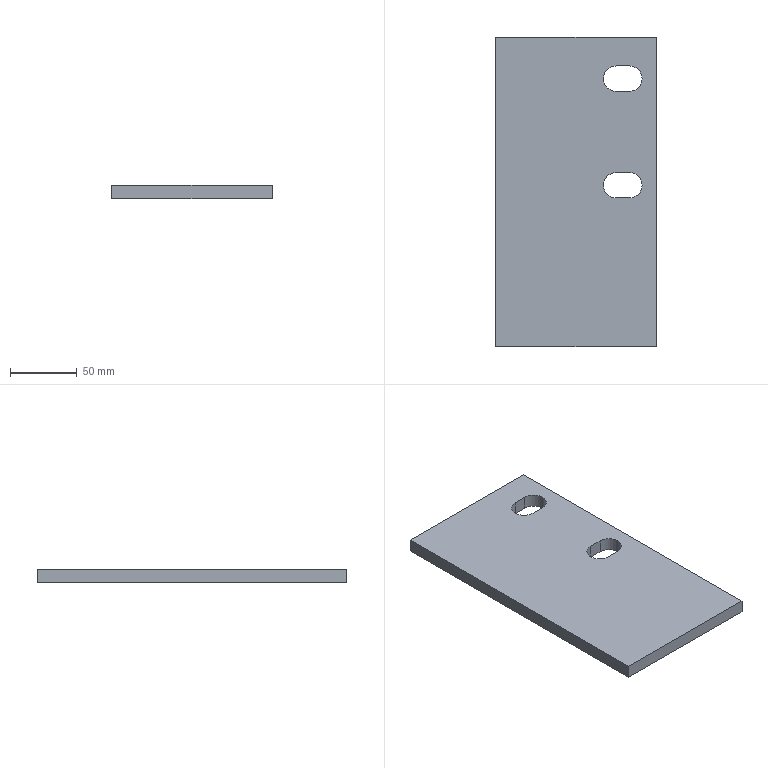Part | STEP file | 粉仓楼梯支撑Plate | 1 solid | 16 faces | box 120 x 232 x 10 mm | volume 268929 mm3 | plane 10 | cylinder 6 | commonest cylinder face diameters 19 x6
STEP:
#1=CARTESIAN_POINT('',(0.,0.,0.));
#2=DIRECTION('',(0.,0.,1.));
#3=DIRECTION('',(1.,0.,0.));
#4=AXIS2_PLACEMENT_3D('',#1,#2,#3);
#5=CARTESIAN_POINT('',(40.,94.5,0.));
#6=VERTEX_POINT('',#5);
#7=CARTESIAN_POINT('',(40.,94.5,10.));
#8=VERTEX_POINT('',#7);
#9=CARTESIAN_POINT('',(40.,94.5,10.));
#10=DIRECTION('',(0.,0.,1.));
#11=VECTOR('',#10,1.);
#12=LINE('',#9,#11);
#13=CARTESIAN_POINT('',(40.,85.,10.));
#14=DIRECTION('',(0.,0.,1.));
#15=DIRECTION('',(1.,0.,0.));
#16=AXIS2_PLACEMENT_3D('',#13,#14,#15);
#17=CYLINDRICAL_SURFACE('',#16,9.5);
#18=CARTESIAN_POINT('',(1.571,0.));
#19=DIRECTION('',(0.,1.));
#20=VECTOR('',#19,1.);
#21=LINE('',#18,#20);
#22=(GEOMETRIC_REPRESENTATION_CONTEXT(2)PARAMETRIC_REPRESENTATION_CONTEXT()REPRESENTATION_CONTEXT('',''));
#23=DEFINITIONAL_REPRESENTATION('',(#21),#22);
#24=PCURVE('',#17,#23);
#25=CARTESIAN_POINT('',(30.,94.5,10.));
#26=DIRECTION('',(0.,1.,0.));
#27=DIRECTION('',(0.,0.,1.));
#28=AXIS2_PLACEMENT_3D('',#25,#26,#27);
#29=PLANE('',#28);
#30=CARTESIAN_POINT('',(0.,10.));
#31=DIRECTION('',(1.,0.));
#32=VECTOR('',#31,1.);
#33=LINE('',#30,#32);
#34=(GEOMETRIC_REPRESENTATION_CONTEXT(2)PARAMETRIC_REPRESENTATION_CONTEXT()REPRESENTATION_CONTEXT('',''));
#35=DEFINITIONAL_REPRESENTATION('',(#33),#34);
#36=PCURVE('',#29,#35);
#37=SURFACE_CURVE('',#12,(#24,#36),.PCURVE_S1.);
#38=EDGE_CURVE('',#6,#8,#37,.T.);
#39=ORIENTED_EDGE('',*,*,#38,.T.);
#40=CARTESIAN_POINT('',(49.5,85.,10.));
#41=VERTEX_POINT('',#40);
#42=CARTESIAN_POINT('',(40.,85.,10.));
#43=DIRECTION('',(0.,0.,1.));
#44=DIRECTION('',(1.,0.,0.));
#45=AXIS2_PLACEMENT_3D('',#42,#43,#44);
#46=CIRCLE('',#45,9.5);
#47=CARTESIAN_POINT('',(0.,0.));
#48=DIRECTION('',(1.,0.));
#49=VECTOR('',#48,1.);
#50=LINE('',#47,#49);
#51=(GEOMETRIC_REPRESENTATION_CONTEXT(2)PARAMETRIC_REPRESENTATION_CONTEXT()REPRESENTATION_CONTEXT('',''));
#52=DEFINITIONAL_REPRESENTATION('',(#50),#51);
#53=PCURVE('',#17,#52);
#54=CARTESIAN_POINT('',(0.,0.,10.));
#55=DIRECTION('',(0.,0.,1.));
#56=DIRECTION('',(1.,0.,0.));
#57=AXIS2_PLACEMENT_3D('',#54,#55,#56);
#58=PLANE('',#57);
#59=CARTESIAN_POINT('',(40.,85.));
#60=DIRECTION('',(1.,0.));
#61=AXIS2_PLACEMENT_2D('',#59,#60);
#62=CIRCLE('',#61,9.5);
#63=(GEOMETRIC_REPRESENTATION_CONTEXT(2)PARAMETRIC_REPRESENTATION_CONTEXT()REPRESENTATION_CONTEXT('',''));
#64=DEFINITIONAL_REPRESENTATION('',(#62),#63);
#65=PCURVE('',#58,#64);
#66=SURFACE_CURVE('',#46,(#53,#65),.PCURVE_S1.);
#67=EDGE_CURVE('',#41,#8,#66,.T.);
#68=ORIENTED_EDGE('',*,*,#67,.F.);
#69=CARTESIAN_POINT('',(49.5,85.,0.));
#70=VERTEX_POINT('',#69);
#71=CARTESIAN_POINT('',(49.5,85.,10.));
#72=DIRECTION('',(0.,0.,1.));
#73=VECTOR('',#72,1.);
#74=LINE('',#71,#73);
#75=CARTESIAN_POINT('',(0.,0.));
#76=DIRECTION('',(0.,1.));
#77=VECTOR('',#76,1.);
#78=LINE('',#75,#77);
#79=(GEOMETRIC_REPRESENTATION_CONTEXT(2)PARAMETRIC_REPRESENTATION_CONTEXT()REPRESENTATION_CONTEXT('',''));
#80=DEFINITIONAL_REPRESENTATION('',(#78),#79);
#81=PCURVE('',#17,#80);
#82=CARTESIAN_POINT('',(40.,85.,10.));
#83=DIRECTION('',(0.,0.,1.));
#84=DIRECTION('',(1.,0.,0.));
#85=AXIS2_PLACEMENT_3D('',#82,#83,#84);
#86=CYLINDRICAL_SURFACE('',#85,9.5);
#87=CARTESIAN_POINT('',(6.283,0.));
#88=DIRECTION('',(0.,1.));
#89=VECTOR('',#88,1.);
#90=LINE('',#87,#89);
#91=(GEOMETRIC_REPRESENTATION_CONTEXT(2)PARAMETRIC_REPRESENTATION_CONTEXT()REPRESENTATION_CONTEXT('',''));
#92=DEFINITIONAL_REPRESENTATION('',(#90),#91);
#93=PCURVE('',#86,#92);
#94=SURFACE_CURVE('',#74,(#81,#93),.PCURVE_S1.);
#95=EDGE_CURVE('',#70,#41,#94,.T.);
#96=ORIENTED_EDGE('',*,*,#95,.F.);
#97=CARTESIAN_POINT('',(40.,85.,0.));
#98=DIRECTION('',(0.,0.,1.));
#99=DIRECTION('',(1.,0.,0.));
#100=AXIS2_PLACEMENT_3D('',#97,#98,#99);
#101=CIRCLE('',#100,9.5);
#102=CARTESIAN_POINT('',(0.,-10.));
#103=DIRECTION('',(1.,0.));
#104=VECTOR('',#103,1.);
#105=LINE('',#102,#104);
#106=(GEOMETRIC_REPRESENTATION_CONTEXT(2)PARAMETRIC_REPRESENTATION_CONTEXT()REPRESENTATION_CONTEXT('',''));
#107=DEFINITIONAL_REPRESENTATION('',(#105),#106);
#108=PCURVE('',#17,#107);
#109=CARTESIAN_POINT('',(0.,0.,0.));
#110=DIRECTION('',(0.,0.,1.));
#111=DIRECTION('',(1.,0.,0.));
#112=AXIS2_PLACEMENT_3D('',#109,#110,#111);
#113=PLANE('',#112);
#114=CARTESIAN_POINT('',(40.,85.));
#115=DIRECTION('',(1.,0.));
#116=AXIS2_PLACEMENT_2D('',#114,#115);
#117=CIRCLE('',#116,9.5);
#118=(GEOMETRIC_REPRESENTATION_CONTEXT(2)PARAMETRIC_REPRESENTATION_CONTEXT()REPRESENTATION_CONTEXT('',''));
#119=DEFINITIONAL_REPRESENTATION('',(#117),#118);
#120=PCURVE('',#113,#119);
#121=SURFACE_CURVE('',#101,(#108,#120),.PCURVE_S1.);
#122=EDGE_CURVE('',#70,#6,#121,.T.);
#123=ORIENTED_EDGE('',*,*,#122,.T.);
#124=EDGE_LOOP('',(#39,#68,#96,#123));
#125=FACE_BOUND('',#124,.F.);
#126=ADVANCED_FACE('',(#125),#17,.F.);
#127=CARTESIAN_POINT('',(40.,14.5,0.));
#128=VERTEX_POINT('',#127);
#129=CARTESIAN_POINT('',(40.,14.5,10.));
#130=VERTEX_POINT('',#129);
#131=CARTESIAN_POINT('',(40.,14.5,10.));
#132=DIRECTION('',(0.,0.,1.));
#133=VECTOR('',#132,1.);
#134=LINE('',#131,#133);
#135=CARTESIAN_POINT('',(40.,5.,10.));
#136=DIRECTION('',(0.,0.,1.));
#137=DIRECTION('',(1.,0.,0.));
#138=AXIS2_PLACEMENT_3D('',#135,#136,#137);
#139=CYLINDRICAL_SURFACE('',#138,9.5);
#140=CARTESIAN_POINT('',(1.571,0.));
#141=DIRECTION('',(0.,1.));
#142=VECTOR('',#141,1.);
#143=LINE('',#140,#142);
#144=(GEOMETRIC_REPRESENTATION_CONTEXT(2)PARAMETRIC_REPRESENTATION_CONTEXT()REPRESENTATION_CONTEXT('',''));
#145=DEFINITIONAL_REPRESENTATION('',(#143),#144);
#146=PCURVE('',#139,#145);
#147=CARTESIAN_POINT('',(30.,14.5,10.));
#148=DIRECTION('',(0.,1.,0.));
#149=DIRECTION('',(0.,0.,1.));
#150=AXIS2_PLACEMENT_3D('',#147,#148,#149);
#151=PLANE('',#150);
#152=CARTESIAN_POINT('',(0.,10.));
#153=DIRECTION('',(1.,0.));
#154=VECTOR('',#153,1.);
#155=LINE('',#152,#154);
#156=(GEOMETRIC_REPRESENTATION_CONTEXT(2)PARAMETRIC_REPRESENTATION_CONTEXT()REPRESENTATION_CONTEXT('',''));
#157=DEFINITIONAL_REPRESENTATION('',(#155),#156);
#158=PCURVE('',#151,#157);
#159=SURFACE_CURVE('',#134,(#146,#158),.PCURVE_S1.);
#160=EDGE_CURVE('',#128,#130,#159,.T.);
#161=ORIENTED_EDGE('',*,*,#160,.T.);
#162=CARTESIAN_POINT('',(49.5,5.,10.));
#163=VERTEX_POINT('',#162);
#164=CARTESIAN_POINT('',(40.,5.,10.));
#165=DIRECTION('',(0.,0.,1.));
#166=DIRECTION('',(1.,0.,0.));
#167=AXIS2_PLACEMENT_3D('',#164,#165,#166);
#168=CIRCLE('',#167,9.5);
#169=CARTESIAN_POINT('',(0.,0.));
#170=DIRECTION('',(1.,0.));
#171=VECTOR('',#170,1.);
#172=LINE('',#169,#171);
#173=(GEOMETRIC_REPRESENTATION_CONTEXT(2)PARAMETRIC_REPRESENTATION_CONTEXT()REPRESENTATION_CONTEXT('',''));
#174=DEFINITIONAL_REPRESENTATION('',(#172),#173);
#175=PCURVE('',#139,#174);
#176=CARTESIAN_POINT('',(40.,5.));
#177=DIRECTION('',(1.,0.));
#178=AXIS2_PLACEMENT_2D('',#176,#177);
#179=CIRCLE('',#178,9.5);
#180=(GEOMETRIC_REPRESENTATION_CONTEXT(2)PARAMETRIC_REPRESENTATION_CONTEXT()REPRESENTATION_CONTEXT('',''));
#181=DEFINITIONAL_REPRESENTATION('',(#179),#180);
#182=PCURVE('',#58,#181);
#183=SURFACE_CURVE('',#168,(#175,#182),.PCURVE_S1.);
#184=EDGE_CURVE('',#163,#130,#183,.T.);
#185=ORIENTED_EDGE('',*,*,#184,.F.);
#186=CARTESIAN_POINT('',(49.5,5.,0.));
#187=VERTEX_POINT('',#186);
#188=CARTESIAN_POINT('',(49.5,5.,10.));
#189=DIRECTION('',(0.,0.,1.));
#190=VECTOR('',#189,1.);
#191=LINE('',#188,#190);
#192=CARTESIAN_POINT('',(0.,0.));
#193=DIRECTION('',(0.,1.));
#194=VECTOR('',#193,1.);
#195=LINE('',#192,#194);
#196=(GEOMETRIC_REPRESENTATION_CONTEXT(2)PARAMETRIC_REPRESENTATION_CONTEXT()REPRESENTATION_CONTEXT('',''));
#197=DEFINITIONAL_REPRESENTATION('',(#195),#196);
#198=PCURVE('',#139,#197);
#199=CARTESIAN_POINT('',(40.,5.,10.));
#200=DIRECTION('',(0.,0.,1.));
#201=DIRECTION('',(1.,0.,0.));
#202=AXIS2_PLACEMENT_3D('',#199,#200,#201);
#203=CYLINDRICAL_SURFACE('',#202,9.5);
#204=CARTESIAN_POINT('',(6.283,0.));
#205=DIRECTION('',(0.,1.));
#206=VECTOR('',#205,1.);
#207=LINE('',#204,#206);
#208=(GEOMETRIC_REPRESENTATION_CONTEXT(2)PARAMETRIC_REPRESENTATION_CONTEXT()REPRESENTATION_CONTEXT('',''));
#209=DEFINITIONAL_REPRESENTATION('',(#207),#208);
#210=PCURVE('',#203,#209);
#211=SURFACE_CURVE('',#191,(#198,#210),.PCURVE_S1.);
#212=EDGE_CURVE('',#187,#163,#211,.T.);
#213=ORIENTED_EDGE('',*,*,#212,.F.);
#214=CARTESIAN_POINT('',(40.,5.,0.));
#215=DIRECTION('',(0.,0.,1.));
#216=DIRECTION('',(1.,0.,0.));
#217=AXIS2_PLACEMENT_3D('',#214,#215,#216);
#218=CIRCLE('',#217,9.5);
#219=CARTESIAN_POINT('',(0.,-10.));
#220=DIRECTION('',(1.,0.));
#221=VECTOR('',#220,1.);
#222=LINE('',#219,#221);
#223=(GEOMETRIC_REPRESENTATION_CONTEXT(2)PARAMETRIC_REPRESENTATION_CONTEXT()REPRESENTATION_CONTEXT('',''));
#224=DEFINITIONAL_REPRESENTATION('',(#222),#223);
#225=PCURVE('',#139,#224);
#226=CARTESIAN_POINT('',(40.,5.));
#227=DIRECTION('',(1.,0.));
#228=AXIS2_PLACEMENT_2D('',#226,#227);
#229=CIRCLE('',#228,9.5);
#230=(GEOMETRIC_REPRESENTATION_CONTEXT(2)PARAMETRIC_REPRESENTATION_CONTEXT()REPRESENTATION_CONTEXT('',''));
#231=DEFINITIONAL_REPRESENTATION('',(#229),#230);
#232=PCURVE('',#113,#231);
#233=SURFACE_CURVE('',#218,(#225,#232),.PCURVE_S1.);
#234=EDGE_CURVE('',#187,#128,#233,.T.);
#235=ORIENTED_EDGE('',*,*,#234,.T.);
#236=EDGE_LOOP('',(#161,#185,#213,#235));
#237=FACE_BOUND('',#236,.F.);
#238=ADVANCED_FACE('',(#237),#139,.F.);
#239=CARTESIAN_POINT('',(60.,-116.,0.));
#240=VERTEX_POINT('',#239);
#241=CARTESIAN_POINT('',(60.,116.,0.));
#242=VERTEX_POINT('',#241);
#243=CARTESIAN_POINT('',(60.,116.,0.));
#244=DIRECTION('',(0.,1.,0.));
#245=VECTOR('',#244,1.);
#246=LINE('',#243,#245);
#247=CARTESIAN_POINT('',(60.,116.,10.));
#248=DIRECTION('',(-1.,0.,0.));
#249=DIRECTION('',(0.,-1.,0.));
#250=AXIS2_PLACEMENT_3D('',#247,#248,#249);
#251=PLANE('',#250);
#252=CARTESIAN_POINT('',(0.,-10.));
#253=DIRECTION('',(-1.,0.));
#254=VECTOR('',#253,1.);
#255=LINE('',#252,#254);
#256=(GEOMETRIC_REPRESENTATION_CONTEXT(2)PARAMETRIC_REPRESENTATION_CONTEXT()REPRESENTATION_CONTEXT('',''));
#257=DEFINITIONAL_REPRESENTATION('',(#255),#256);
#258=PCURVE('',#251,#257);
#259=CARTESIAN_POINT('',(60.,116.));
#260=DIRECTION('',(0.,1.));
#261=VECTOR('',#260,1.);
#262=LINE('',#259,#261);
#263=(GEOMETRIC_REPRESENTATION_CONTEXT(2)PARAMETRIC_REPRESENTATION_CONTEXT()REPRESENTATION_CONTEXT('',''));
#264=DEFINITIONAL_REPRESENTATION('',(#262),#263);
#265=PCURVE('',#113,#264);
#266=SURFACE_CURVE('',#246,(#258,#265),.PCURVE_S1.);
#267=EDGE_CURVE('',#240,#242,#266,.T.);
#268=ORIENTED_EDGE('',*,*,#267,.T.);
#269=CARTESIAN_POINT('',(60.,116.,10.));
#270=VERTEX_POINT('',#269);
#271=CARTESIAN_POINT('',(60.,116.,10.));
#272=DIRECTION('',(0.,0.,-1.));
#273=VECTOR('',#272,1.);
#274=LINE('',#271,#273);
#275=CARTESIAN_POINT('',(0.,0.));
#276=DIRECTION('',(0.,-1.));
#277=VECTOR('',#276,1.);
#278=LINE('',#275,#277);
#279=(GEOMETRIC_REPRESENTATION_CONTEXT(2)PARAMETRIC_REPRESENTATION_CONTEXT()REPRESENTATION_CONTEXT('',''));
#280=DEFINITIONAL_REPRESENTATION('',(#278),#279);
#281=PCURVE('',#251,#280);
#282=CARTESIAN_POINT('',(-60.,116.,10.));
#283=DIRECTION('',(0.,-1.,0.));
#284=DIRECTION('',(1.,0.,0.));
#285=AXIS2_PLACEMENT_3D('',#282,#283,#284);
#286=PLANE('',#285);
#287=CARTESIAN_POINT('',(120.,0.));
#288=DIRECTION('',(0.,-1.));
#289=VECTOR('',#288,1.);
#290=LINE('',#287,#289);
#291=(GEOMETRIC_REPRESENTATION_CONTEXT(2)PARAMETRIC_REPRESENTATION_CONTEXT()REPRESENTATION_CONTEXT('',''));
#292=DEFINITIONAL_REPRESENTATION('',(#290),#291);
#293=PCURVE('',#286,#292);
#294=SURFACE_CURVE('',#274,(#281,#293),.PCURVE_S1.);
#295=EDGE_CURVE('',#270,#242,#294,.T.);
#296=ORIENTED_EDGE('',*,*,#295,.F.);
#297=CARTESIAN_POINT('',(60.,-116.,10.));
#298=VERTEX_POINT('',#297);
#299=CARTESIAN_POINT('',(60.,116.,10.));
#300=DIRECTION('',(0.,1.,0.));
#301=VECTOR('',#300,1.);
#302=LINE('',#299,#301);
#303=CARTESIAN_POINT('',(0.,0.));
#304=DIRECTION('',(-1.,0.));
#305=VECTOR('',#304,1.);
#306=LINE('',#303,#305);
#307=(GEOMETRIC_REPRESENTATION_CONTEXT(2)PARAMETRIC_REPRESENTATION_CONTEXT()REPRESENTATION_CONTEXT('',''));
#308=DEFINITIONAL_REPRESENTATION('',(#306),#307);
#309=PCURVE('',#251,#308);
#310=CARTESIAN_POINT('',(60.,116.));
#311=DIRECTION('',(0.,1.));
#312=VECTOR('',#311,1.);
#313=LINE('',#310,#312);
#314=(GEOMETRIC_REPRESENTATION_CONTEXT(2)PARAMETRIC_REPRESENTATION_CONTEXT()REPRESENTATION_CONTEXT('',''));
#315=DEFINITIONAL_REPRESENTATION('',(#313),#314);
#316=PCURVE('',#58,#315);
#317=SURFACE_CURVE('',#302,(#309,#316),.PCURVE_S1.);
#318=EDGE_CURVE('',#298,#270,#317,.T.);
#319=ORIENTED_EDGE('',*,*,#318,.F.);
#320=CARTESIAN_POINT('',(60.,-116.,10.));
#321=DIRECTION('',(0.,0.,-1.));
#322=VECTOR('',#321,1.);
#323=LINE('',#320,#322);
#324=CARTESIAN_POINT('',(232.,0.));
#325=DIRECTION('',(0.,-1.));
#326=VECTOR('',#325,1.);
#327=LINE('',#324,#326);
#328=(GEOMETRIC_REPRESENTATION_CONTEXT(2)PARAMETRIC_REPRESENTATION_CONTEXT()REPRESENTATION_CONTEXT('',''));
#329=DEFINITIONAL_REPRESENTATION('',(#327),#328);
#330=PCURVE('',#251,#329);
#331=CARTESIAN_POINT('',(-60.,-116.,10.));
#332=DIRECTION('',(0.,1.,0.));
#333=DIRECTION('',(0.,0.,1.));
#334=AXIS2_PLACEMENT_3D('',#331,#332,#333);
#335=PLANE('',#334);
#336=CARTESIAN_POINT('',(0.,120.));
#337=DIRECTION('',(-1.,0.));
#338=VECTOR('',#337,1.);
#339=LINE('',#336,#338);
#340=(GEOMETRIC_REPRESENTATION_CONTEXT(2)PARAMETRIC_REPRESENTATION_CONTEXT()REPRESENTATION_CONTEXT('',''));
#341=DEFINITIONAL_REPRESENTATION('',(#339),#340);
#342=PCURVE('',#335,#341);
#343=SURFACE_CURVE('',#323,(#330,#342),.PCURVE_S1.);
#344=EDGE_CURVE('',#298,#240,#343,.T.);
#345=ORIENTED_EDGE('',*,*,#344,.T.);
#346=EDGE_LOOP('',(#268,#296,#319,#345));
#347=FACE_BOUND('',#346,.T.);
#348=ADVANCED_FACE('',(#347),#251,.F.);
#349=CARTESIAN_POINT('',(-60.,116.,0.));
#350=VERTEX_POINT('',#349);
#351=CARTESIAN_POINT('',(-60.,116.,0.));
#352=DIRECTION('',(-1.,0.,0.));
#353=VECTOR('',#352,1.);
#354=LINE('',#351,#353);
#355=CARTESIAN_POINT('',(0.,-10.));
#356=DIRECTION('',(-1.,0.));
#357=VECTOR('',#356,1.);
#358=LINE('',#355,#357);
#359=(GEOMETRIC_REPRESENTATION_CONTEXT(2)PARAMETRIC_REPRESENTATION_CONTEXT()REPRESENTATION_CONTEXT('',''));
#360=DEFINITIONAL_REPRESENTATION('',(#358),#359);
#361=PCURVE('',#286,#360);
#362=CARTESIAN_POINT('',(-60.,116.));
#363=DIRECTION('',(-1.,0.));
#364=VECTOR('',#363,1.);
#365=LINE('',#362,#364);
#366=(GEOMETRIC_REPRESENTATION_CONTEXT(2)PARAMETRIC_REPRESENTATION_CONTEXT()REPRESENTATION_CONTEXT('',''));
#367=DEFINITIONAL_REPRESENTATION('',(#365),#366);
#368=PCURVE('',#113,#367);
#369=SURFACE_CURVE('',#354,(#361,#368),.PCURVE_S1.);
#370=EDGE_CURVE('',#242,#350,#369,.T.);
#371=ORIENTED_EDGE('',*,*,#370,.T.);
#372=CARTESIAN_POINT('',(-60.,116.,10.));
#373=VERTEX_POINT('',#372);
#374=CARTESIAN_POINT('',(-60.,116.,10.));
#375=DIRECTION('',(0.,0.,-1.));
#376=VECTOR('',#375,1.);
#377=LINE('',#374,#376);
#378=CARTESIAN_POINT('',(0.,0.));
#379=DIRECTION('',(0.,-1.));
#380=VECTOR('',#379,1.);
#381=LINE('',#378,#380);
#382=(GEOMETRIC_REPRESENTATION_CONTEXT(2)PARAMETRIC_REPRESENTATION_CONTEXT()REPRESENTATION_CONTEXT('',''));
#383=DEFINITIONAL_REPRESENTATION('',(#381),#382);
#384=PCURVE('',#286,#383);
#385=CARTESIAN_POINT('',(-60.,116.,10.));
#386=DIRECTION('',(1.,0.,0.));
#387=DIRECTION('',(0.,1.,0.));
#388=AXIS2_PLACEMENT_3D('',#385,#386,#387);
#389=PLANE('',#388);
#390=CARTESIAN_POINT('',(0.,0.));
#391=DIRECTION('',(0.,-1.));
#392=VECTOR('',#391,1.);
#393=LINE('',#390,#392);
#394=(GEOMETRIC_REPRESENTATION_CONTEXT(2)PARAMETRIC_REPRESENTATION_CONTEXT()REPRESENTATION_CONTEXT('',''));
#395=DEFINITIONAL_REPRESENTATION('',(#393),#394);
#396=PCURVE('',#389,#395);
#397=SURFACE_CURVE('',#377,(#384,#396),.PCURVE_S1.);
#398=EDGE_CURVE('',#373,#350,#397,.T.);
#399=ORIENTED_EDGE('',*,*,#398,.F.);
#400=CARTESIAN_POINT('',(-60.,116.,10.));
#401=DIRECTION('',(-1.,0.,0.));
#402=VECTOR('',#401,1.);
#403=LINE('',#400,#402);
#404=CARTESIAN_POINT('',(0.,0.));
#405=DIRECTION('',(-1.,0.));
#406=VECTOR('',#405,1.);
#407=LINE('',#404,#406);
#408=(GEOMETRIC_REPRESENTATION_CONTEXT(2)PARAMETRIC_REPRESENTATION_CONTEXT()REPRESENTATION_CONTEXT('',''));
#409=DEFINITIONAL_REPRESENTATION('',(#407),#408);
#410=PCURVE('',#286,#409);
#411=CARTESIAN_POINT('',(-60.,116.));
#412=DIRECTION('',(-1.,0.));
#413=VECTOR('',#412,1.);
#414=LINE('',#411,#413);
#415=(GEOMETRIC_REPRESENTATION_CONTEXT(2)PARAMETRIC_REPRESENTATION_CONTEXT()REPRESENTATION_CONTEXT('',''));
#416=DEFINITIONAL_REPRESENTATION('',(#414),#415);
#417=PCURVE('',#58,#416);
#418=SURFACE_CURVE('',#403,(#410,#417),.PCURVE_S1.);
#419=EDGE_CURVE('',#270,#373,#418,.T.);
#420=ORIENTED_EDGE('',*,*,#419,.F.);
#421=ORIENTED_EDGE('',*,*,#295,.T.);
#422=EDGE_LOOP('',(#371,#399,#420,#421));
#423=FACE_BOUND('',#422,.T.);
#424=ADVANCED_FACE('',(#423),#286,.F.);
#425=CARTESIAN_POINT('',(-60.,-116.,0.));
#426=VERTEX_POINT('',#425);
#427=CARTESIAN_POINT('',(-60.,116.,0.));
#428=DIRECTION('',(0.,-1.,0.));
#429=VECTOR('',#428,1.);
#430=LINE('',#427,#429);
#431=CARTESIAN_POINT('',(0.,-10.));
#432=DIRECTION('',(-1.,0.));
#433=VECTOR('',#432,1.);
#434=LINE('',#431,#433);
#435=(GEOMETRIC_REPRESENTATION_CONTEXT(2)PARAMETRIC_REPRESENTATION_CONTEXT()REPRESENTATION_CONTEXT('',''));
#436=DEFINITIONAL_REPRESENTATION('',(#434),#435);
#437=PCURVE('',#389,#436);
#438=CARTESIAN_POINT('',(-60.,116.));
#439=DIRECTION('',(0.,-1.));
#440=VECTOR('',#439,1.);
#441=LINE('',#438,#440);
#442=(GEOMETRIC_REPRESENTATION_CONTEXT(2)PARAMETRIC_REPRESENTATION_CONTEXT()REPRESENTATION_CONTEXT('',''));
#443=DEFINITIONAL_REPRESENTATION('',(#441),#442);
#444=PCURVE('',#113,#443);
#445=SURFACE_CURVE('',#430,(#437,#444),.PCURVE_S1.);
#446=EDGE_CURVE('',#350,#426,#445,.T.);
#447=ORIENTED_EDGE('',*,*,#446,.T.);
#448=CARTESIAN_POINT('',(-60.,-116.,10.));
#449=VERTEX_POINT('',#448);
#450=CARTESIAN_POINT('',(-60.,-116.,10.));
#451=DIRECTION('',(0.,0.,-1.));
#452=VECTOR('',#451,1.);
#453=LINE('',#450,#452);
#454=CARTESIAN_POINT('',(-232.,0.));
#455=DIRECTION('',(0.,-1.));
#456=VECTOR('',#455,1.);
#457=LINE('',#454,#456);
#458=(GEOMETRIC_REPRESENTATION_CONTEXT(2)PARAMETRIC_REPRESENTATION_CONTEXT()REPRESENTATION_CONTEXT('',''));
#459=DEFINITIONAL_REPRESENTATION('',(#457),#458);
#460=PCURVE('',#389,#459);
#461=CARTESIAN_POINT('',(0.,0.));
#462=DIRECTION('',(-1.,0.));
#463=VECTOR('',#462,1.);
#464=LINE('',#461,#463);
#465=(GEOMETRIC_REPRESENTATION_CONTEXT(2)PARAMETRIC_REPRESENTATION_CONTEXT()REPRESENTATION_CONTEXT('',''));
#466=DEFINITIONAL_REPRESENTATION('',(#464),#465);
#467=PCURVE('',#335,#466);
#468=SURFACE_CURVE('',#453,(#460,#467),.PCURVE_S1.);
#469=EDGE_CURVE('',#449,#426,#468,.T.);
#470=ORIENTED_EDGE('',*,*,#469,.F.);
#471=CARTESIAN_POINT('',(-60.,116.,10.));
#472=DIRECTION('',(0.,-1.,0.));
#473=VECTOR('',#472,1.);
#474=LINE('',#471,#473);
#475=CARTESIAN_POINT('',(0.,0.));
#476=DIRECTION('',(-1.,0.));
#477=VECTOR('',#476,1.);
#478=LINE('',#475,#477);
#479=(GEOMETRIC_REPRESENTATION_CONTEXT(2)PARAMETRIC_REPRESENTATION_CONTEXT()REPRESENTATION_CONTEXT('',''));
#480=DEFINITIONAL_REPRESENTATION('',(#478),#479);
#481=PCURVE('',#389,#480);
#482=CARTESIAN_POINT('',(-60.,116.));
#483=DIRECTION('',(0.,-1.));
#484=VECTOR('',#483,1.);
#485=LINE('',#482,#484);
#486=(GEOMETRIC_REPRESENTATION_CONTEXT(2)PARAMETRIC_REPRESENTATION_CONTEXT()REPRESENTATION_CONTEXT('',''));
#487=DEFINITIONAL_REPRESENTATION('',(#485),#486);
#488=PCURVE('',#58,#487);
#489=SURFACE_CURVE('',#474,(#481,#488),.PCURVE_S1.);
#490=EDGE_CURVE('',#373,#449,#489,.T.);
#491=ORIENTED_EDGE('',*,*,#490,.F.);
#492=ORIENTED_EDGE('',*,*,#398,.T.);
#493=EDGE_LOOP('',(#447,#470,#491,#492));
#494=FACE_BOUND('',#493,.T.);
#495=ADVANCED_FACE('',(#494),#389,.F.);
#496=CARTESIAN_POINT('',(-60.,-116.,0.));
#497=DIRECTION('',(1.,0.,0.));
#498=VECTOR('',#497,1.);
#499=LINE('',#496,#498);
#500=CARTESIAN_POINT('',(-10.,0.));
#501=DIRECTION('',(0.,1.));
#502=VECTOR('',#501,1.);
#503=LINE('',#500,#502);
#504=(GEOMETRIC_REPRESENTATION_CONTEXT(2)PARAMETRIC_REPRESENTATION_CONTEXT()REPRESENTATION_CONTEXT('',''));
#505=DEFINITIONAL_REPRESENTATION('',(#503),#504);
#506=PCURVE('',#335,#505);
#507=CARTESIAN_POINT('',(-60.,-116.));
#508=DIRECTION('',(1.,0.));
#509=VECTOR('',#508,1.);
#510=LINE('',#507,#509);
#511=(GEOMETRIC_REPRESENTATION_CONTEXT(2)PARAMETRIC_REPRESENTATION_CONTEXT()REPRESENTATION_CONTEXT('',''));
#512=DEFINITIONAL_REPRESENTATION('',(#510),#511);
#513=PCURVE('',#113,#512);
#514=SURFACE_CURVE('',#499,(#506,#513),.PCURVE_S1.);
#515=EDGE_CURVE('',#426,#240,#514,.T.);
#516=ORIENTED_EDGE('',*,*,#515,.T.);
#517=ORIENTED_EDGE('',*,*,#344,.F.);
#518=CARTESIAN_POINT('',(-60.,-116.,10.));
#519=DIRECTION('',(1.,0.,0.));
#520=VECTOR('',#519,1.);
#521=LINE('',#518,#520);
#522=CARTESIAN_POINT('',(0.,0.));
#523=DIRECTION('',(0.,1.));
#524=VECTOR('',#523,1.);
#525=LINE('',#522,#524);
#526=(GEOMETRIC_REPRESENTATION_CONTEXT(2)PARAMETRIC_REPRESENTATION_CONTEXT()REPRESENTATION_CONTEXT('',''));
#527=DEFINITIONAL_REPRESENTATION('',(#525),#526);
#528=PCURVE('',#335,#527);
#529=CARTESIAN_POINT('',(-60.,-116.));
#530=DIRECTION('',(1.,0.));
#531=VECTOR('',#530,1.);
#532=LINE('',#529,#531);
#533=(GEOMETRIC_REPRESENTATION_CONTEXT(2)PARAMETRIC_REPRESENTATION_CONTEXT()REPRESENTATION_CONTEXT('',''));
#534=DEFINITIONAL_REPRESENTATION('',(#532),#533);
#535=PCURVE('',#58,#534);
#536=SURFACE_CURVE('',#521,(#528,#535),.PCURVE_S1.);
#537=EDGE_CURVE('',#449,#298,#536,.T.);
#538=ORIENTED_EDGE('',*,*,#537,.F.);
#539=ORIENTED_EDGE('',*,*,#469,.T.);
#540=EDGE_LOOP('',(#516,#517,#538,#539));
#541=FACE_BOUND('',#540,.T.);
#542=ADVANCED_FACE('',(#541),#335,.F.);
#543=CARTESIAN_POINT('',(30.,94.5,10.));
#544=VERTEX_POINT('',#543);
#545=CARTESIAN_POINT('',(30.,75.5,10.));
#546=VERTEX_POINT('',#545);
#547=CARTESIAN_POINT('',(30.,85.,10.));
#548=DIRECTION('',(0.,0.,1.));
#549=DIRECTION('',(1.,0.,0.));
#550=AXIS2_PLACEMENT_3D('',#547,#548,#549);
#551=CIRCLE('',#550,9.5);
#552=CARTESIAN_POINT('',(30.,85.));
#553=DIRECTION('',(1.,0.));
#554=AXIS2_PLACEMENT_2D('',#552,#553);
#555=CIRCLE('',#554,9.5);
#556=(GEOMETRIC_REPRESENTATION_CONTEXT(2)PARAMETRIC_REPRESENTATION_CONTEXT()REPRESENTATION_CONTEXT('',''));
#557=DEFINITIONAL_REPRESENTATION('',(#555),#556);
#558=PCURVE('',#58,#557);
#559=CARTESIAN_POINT('',(30.,85.,10.));
#560=DIRECTION('',(0.,0.,1.));
#561=DIRECTION('',(1.,0.,0.));
#562=AXIS2_PLACEMENT_3D('',#559,#560,#561);
#563=CYLINDRICAL_SURFACE('',#562,9.5);
#564=CARTESIAN_POINT('',(0.,0.));
#565=DIRECTION('',(1.,0.));
#566=VECTOR('',#565,1.);
#567=LINE('',#564,#566);
#568=(GEOMETRIC_REPRESENTATION_CONTEXT(2)PARAMETRIC_REPRESENTATION_CONTEXT()REPRESENTATION_CONTEXT('',''));
#569=DEFINITIONAL_REPRESENTATION('',(#567),#568);
#570=PCURVE('',#563,#569);
#571=SURFACE_CURVE('',#551,(#558,#570),.PCURVE_S1.);
#572=EDGE_CURVE('',#544,#546,#571,.T.);
#573=ORIENTED_EDGE('',*,*,#572,.F.);
#574=CARTESIAN_POINT('',(30.,94.5,10.));
#575=DIRECTION('',(1.,0.,0.));
#576=VECTOR('',#575,1.);
#577=LINE('',#574,#576);
#578=CARTESIAN_POINT('',(30.,94.5));
#579=DIRECTION('',(1.,0.));
#580=VECTOR('',#579,1.);
#581=LINE('',#578,#580);
#582=(GEOMETRIC_REPRESENTATION_CONTEXT(2)PARAMETRIC_REPRESENTATION_CONTEXT()REPRESENTATION_CONTEXT('',''));
#583=DEFINITIONAL_REPRESENTATION('',(#581),#582);
#584=PCURVE('',#58,#583);
#585=CARTESIAN_POINT('',(0.,0.));
#586=DIRECTION('',(0.,1.));
#587=VECTOR('',#586,1.);
#588=LINE('',#585,#587);
#589=(GEOMETRIC_REPRESENTATION_CONTEXT(2)PARAMETRIC_REPRESENTATION_CONTEXT()REPRESENTATION_CONTEXT('',''));
#590=DEFINITIONAL_REPRESENTATION('',(#588),#589);
#591=PCURVE('',#29,#590);
#592=SURFACE_CURVE('',#577,(#584,#591),.PCURVE_S1.);
#593=EDGE_CURVE('',#544,#8,#592,.T.);
#594=ORIENTED_EDGE('',*,*,#593,.T.);
#595=ORIENTED_EDGE('',*,*,#67,.F.);
#596=CARTESIAN_POINT('',(40.,75.5,10.));
#597=VERTEX_POINT('',#596);
#598=CARTESIAN_POINT('',(40.,85.,10.));
#599=DIRECTION('',(0.,0.,1.));
#600=DIRECTION('',(1.,0.,0.));
#601=AXIS2_PLACEMENT_3D('',#598,#599,#600);
#602=CIRCLE('',#601,9.5);
#603=CARTESIAN_POINT('',(40.,85.));
#604=DIRECTION('',(1.,0.));
#605=AXIS2_PLACEMENT_2D('',#603,#604);
#606=CIRCLE('',#605,9.5);
#607=(GEOMETRIC_REPRESENTATION_CONTEXT(2)PARAMETRIC_REPRESENTATION_CONTEXT()REPRESENTATION_CONTEXT('',''));
#608=DEFINITIONAL_REPRESENTATION('',(#606),#607);
#609=PCURVE('',#58,#608);
#610=CARTESIAN_POINT('',(0.,0.));
#611=DIRECTION('',(1.,0.));
#612=VECTOR('',#611,1.);
#613=LINE('',#610,#612);
#614=(GEOMETRIC_REPRESENTATION_CONTEXT(2)PARAMETRIC_REPRESENTATION_CONTEXT()REPRESENTATION_CONTEXT('',''));
#615=DEFINITIONAL_REPRESENTATION('',(#613),#614);
#616=PCURVE('',#86,#615);
#617=SURFACE_CURVE('',#602,(#609,#616),.PCURVE_S1.);
#618=EDGE_CURVE('',#597,#41,#617,.T.);
#619=ORIENTED_EDGE('',*,*,#618,.F.);
#620=CARTESIAN_POINT('',(30.,75.5,10.));
#621=DIRECTION('',(1.,0.,0.));
#622=VECTOR('',#621,1.);
#623=LINE('',#620,#622);
#624=CARTESIAN_POINT('',(30.,75.5));
#625=DIRECTION('',(1.,0.));
#626=VECTOR('',#625,1.);
#627=LINE('',#624,#626);
#628=(GEOMETRIC_REPRESENTATION_CONTEXT(2)PARAMETRIC_REPRESENTATION_CONTEXT()REPRESENTATION_CONTEXT('',''));
#629=DEFINITIONAL_REPRESENTATION('',(#627),#628);
#630=PCURVE('',#58,#629);
#631=CARTESIAN_POINT('',(30.,75.5,10.));
#632=DIRECTION('',(0.,-1.,0.));
#633=DIRECTION('',(0.,0.,-1.));
#634=AXIS2_PLACEMENT_3D('',#631,#632,#633);
#635=PLANE('',#634);
#636=CARTESIAN_POINT('',(0.,0.));
#637=DIRECTION('',(0.,1.));
#638=VECTOR('',#637,1.);
#639=LINE('',#636,#638);
#640=(GEOMETRIC_REPRESENTATION_CONTEXT(2)PARAMETRIC_REPRESENTATION_CONTEXT()REPRESENTATION_CONTEXT('',''));
#641=DEFINITIONAL_REPRESENTATION('',(#639),#640);
#642=PCURVE('',#635,#641);
#643=SURFACE_CURVE('',#623,(#630,#642),.PCURVE_S1.);
#644=EDGE_CURVE('',#546,#597,#643,.T.);
#645=ORIENTED_EDGE('',*,*,#644,.F.);
#646=EDGE_LOOP('',(#573,#594,#595,#619,#645));
#647=FACE_BOUND('',#646,.T.);
#648=CARTESIAN_POINT('',(30.,-4.5,10.));
#649=VERTEX_POINT('',#648);
#650=CARTESIAN_POINT('',(40.,-4.5,10.));
#651=VERTEX_POINT('',#650);
#652=CARTESIAN_POINT('',(30.,-4.5,10.));
#653=DIRECTION('',(1.,0.,0.));
#654=VECTOR('',#653,1.);
#655=LINE('',#652,#654);
#656=CARTESIAN_POINT('',(30.,-4.5));
#657=DIRECTION('',(1.,0.));
#658=VECTOR('',#657,1.);
#659=LINE('',#656,#658);
#660=(GEOMETRIC_REPRESENTATION_CONTEXT(2)PARAMETRIC_REPRESENTATION_CONTEXT()REPRESENTATION_CONTEXT('',''));
#661=DEFINITIONAL_REPRESENTATION('',(#659),#660);
#662=PCURVE('',#58,#661);
#663=CARTESIAN_POINT('',(30.,-4.5,10.));
#664=DIRECTION('',(0.,-1.,0.));
#665=DIRECTION('',(0.,0.,-1.));
#666=AXIS2_PLACEMENT_3D('',#663,#664,#665);
#667=PLANE('',#666);
#668=CARTESIAN_POINT('',(0.,0.));
#669=DIRECTION('',(0.,1.));
#670=VECTOR('',#669,1.);
#671=LINE('',#668,#670);
#672=(GEOMETRIC_REPRESENTATION_CONTEXT(2)PARAMETRIC_REPRESENTATION_CONTEXT()REPRESENTATION_CONTEXT('',''));
#673=DEFINITIONAL_REPRESENTATION('',(#671),#672);
#674=PCURVE('',#667,#673);
#675=SURFACE_CURVE('',#655,(#662,#674),.PCURVE_S1.);
#676=EDGE_CURVE('',#649,#651,#675,.T.);
#677=ORIENTED_EDGE('',*,*,#676,.F.);
#678=CARTESIAN_POINT('',(30.,14.5,10.));
#679=VERTEX_POINT('',#678);
#680=CARTESIAN_POINT('',(30.,5.,10.));
#681=DIRECTION('',(0.,0.,1.));
#682=DIRECTION('',(1.,0.,0.));
#683=AXIS2_PLACEMENT_3D('',#680,#681,#682);
#684=CIRCLE('',#683,9.5);
#685=CARTESIAN_POINT('',(30.,5.));
#686=DIRECTION('',(1.,0.));
#687=AXIS2_PLACEMENT_2D('',#685,#686);
#688=CIRCLE('',#687,9.5);
#689=(GEOMETRIC_REPRESENTATION_CONTEXT(2)PARAMETRIC_REPRESENTATION_CONTEXT()REPRESENTATION_CONTEXT('',''));
#690=DEFINITIONAL_REPRESENTATION('',(#688),#689);
#691=PCURVE('',#58,#690);
#692=CARTESIAN_POINT('',(30.,5.,10.));
#693=DIRECTION('',(0.,0.,1.));
#694=DIRECTION('',(1.,0.,0.));
#695=AXIS2_PLACEMENT_3D('',#692,#693,#694);
#696=CYLINDRICAL_SURFACE('',#695,9.5);
#697=CARTESIAN_POINT('',(0.,0.));
#698=DIRECTION('',(1.,0.));
#699=VECTOR('',#698,1.);
#700=LINE('',#697,#699);
#701=(GEOMETRIC_REPRESENTATION_CONTEXT(2)PARAMETRIC_REPRESENTATION_CONTEXT()REPRESENTATION_CONTEXT('',''));
#702=DEFINITIONAL_REPRESENTATION('',(#700),#701);
#703=PCURVE('',#696,#702);
#704=SURFACE_CURVE('',#684,(#691,#703),.PCURVE_S1.);
#705=EDGE_CURVE('',#679,#649,#704,.T.);
#706=ORIENTED_EDGE('',*,*,#705,.F.);
#707=CARTESIAN_POINT('',(30.,14.5,10.));
#708=DIRECTION('',(1.,0.,0.));
#709=VECTOR('',#708,1.);
#710=LINE('',#707,#709);
#711=CARTESIAN_POINT('',(30.,14.5));
#712=DIRECTION('',(1.,0.));
#713=VECTOR('',#712,1.);
#714=LINE('',#711,#713);
#715=(GEOMETRIC_REPRESENTATION_CONTEXT(2)PARAMETRIC_REPRESENTATION_CONTEXT()REPRESENTATION_CONTEXT('',''));
#716=DEFINITIONAL_REPRESENTATION('',(#714),#715);
#717=PCURVE('',#58,#716);
#718=CARTESIAN_POINT('',(0.,0.));
#719=DIRECTION('',(0.,1.));
#720=VECTOR('',#719,1.);
#721=LINE('',#718,#720);
#722=(GEOMETRIC_REPRESENTATION_CONTEXT(2)PARAMETRIC_REPRESENTATION_CONTEXT()REPRESENTATION_CONTEXT('',''));
#723=DEFINITIONAL_REPRESENTATION('',(#721),#722);
#724=PCURVE('',#151,#723);
#725=SURFACE_CURVE('',#710,(#717,#724),.PCURVE_S1.);
#726=EDGE_CURVE('',#679,#130,#725,.T.);
#727=ORIENTED_EDGE('',*,*,#726,.T.);
#728=ORIENTED_EDGE('',*,*,#184,.F.);
#729=CARTESIAN_POINT('',(40.,5.,10.));
#730=DIRECTION('',(0.,0.,1.));
#731=DIRECTION('',(1.,0.,0.));
#732=AXIS2_PLACEMENT_3D('',#729,#730,#731);
#733=CIRCLE('',#732,9.5);
#734=CARTESIAN_POINT('',(40.,5.));
#735=DIRECTION('',(1.,0.));
#736=AXIS2_PLACEMENT_2D('',#734,#735);
#737=CIRCLE('',#736,9.5);
#738=(GEOMETRIC_REPRESENTATION_CONTEXT(2)PARAMETRIC_REPRESENTATION_CONTEXT()REPRESENTATION_CONTEXT('',''));
#739=DEFINITIONAL_REPRESENTATION('',(#737),#738);
#740=PCURVE('',#58,#739);
#741=CARTESIAN_POINT('',(0.,0.));
#742=DIRECTION('',(1.,0.));
#743=VECTOR('',#742,1.);
#744=LINE('',#741,#743);
#745=(GEOMETRIC_REPRESENTATION_CONTEXT(2)PARAMETRIC_REPRESENTATION_CONTEXT()REPRESENTATION_CONTEXT('',''));
#746=DEFINITIONAL_REPRESENTATION('',(#744),#745);
#747=PCURVE('',#203,#746);
#748=SURFACE_CURVE('',#733,(#740,#747),.PCURVE_S1.);
#749=EDGE_CURVE('',#651,#163,#748,.T.);
#750=ORIENTED_EDGE('',*,*,#749,.F.);
#751=EDGE_LOOP('',(#677,#706,#727,#728,#750));
#752=FACE_BOUND('',#751,.T.);
#753=ORIENTED_EDGE('',*,*,#318,.T.);
#754=ORIENTED_EDGE('',*,*,#419,.T.);
#755=ORIENTED_EDGE('',*,*,#490,.T.);
#756=ORIENTED_EDGE('',*,*,#537,.T.);
#757=EDGE_LOOP('',(#753,#754,#755,#756));
#758=FACE_BOUND('',#757,.T.);
#759=ADVANCED_FACE('',(#647,#752,#758),#58,.T.);
#760=CARTESIAN_POINT('',(30.,94.5,0.));
#761=VERTEX_POINT('',#760);
#762=CARTESIAN_POINT('',(0.,94.5,0.));
#763=DIRECTION('',(-1.,0.,0.));
#764=VECTOR('',#763,1.);
#765=LINE('',#762,#764);
#766=CARTESIAN_POINT('',(0.,94.5));
#767=DIRECTION('',(-1.,0.));
#768=VECTOR('',#767,1.);
#769=LINE('',#766,#768);
#770=(GEOMETRIC_REPRESENTATION_CONTEXT(2)PARAMETRIC_REPRESENTATION_CONTEXT()REPRESENTATION_CONTEXT('',''));
#771=DEFINITIONAL_REPRESENTATION('',(#769),#770);
#772=PCURVE('',#113,#771);
#773=CARTESIAN_POINT('',(-10.,-30.));
#774=DIRECTION('',(0.,-1.));
#775=VECTOR('',#774,1.);
#776=LINE('',#773,#775);
#777=(GEOMETRIC_REPRESENTATION_CONTEXT(2)PARAMETRIC_REPRESENTATION_CONTEXT()REPRESENTATION_CONTEXT('',''));
#778=DEFINITIONAL_REPRESENTATION('',(#776),#777);
#779=PCURVE('',#29,#778);
#780=SURFACE_CURVE('',#765,(#772,#779),.PCURVE_S1.);
#781=EDGE_CURVE('',#6,#761,#780,.T.);
#782=ORIENTED_EDGE('',*,*,#781,.T.);
#783=CARTESIAN_POINT('',(30.,75.5,0.));
#784=VERTEX_POINT('',#783);
#785=CARTESIAN_POINT('',(30.,85.,0.));
#786=DIRECTION('',(0.,0.,1.));
#787=DIRECTION('',(1.,0.,0.));
#788=AXIS2_PLACEMENT_3D('',#785,#786,#787);
#789=CIRCLE('',#788,9.5);
#790=CARTESIAN_POINT('',(30.,85.));
#791=DIRECTION('',(1.,0.));
#792=AXIS2_PLACEMENT_2D('',#790,#791);
#793=CIRCLE('',#792,9.5);
#794=(GEOMETRIC_REPRESENTATION_CONTEXT(2)PARAMETRIC_REPRESENTATION_CONTEXT()REPRESENTATION_CONTEXT('',''));
#795=DEFINITIONAL_REPRESENTATION('',(#793),#794);
#796=PCURVE('',#113,#795);
#797=CARTESIAN_POINT('',(0.,-10.));
#798=DIRECTION('',(1.,0.));
#799=VECTOR('',#798,1.);
#800=LINE('',#797,#799);
#801=(GEOMETRIC_REPRESENTATION_CONTEXT(2)PARAMETRIC_REPRESENTATION_CONTEXT()REPRESENTATION_CONTEXT('',''));
#802=DEFINITIONAL_REPRESENTATION('',(#800),#801);
#803=PCURVE('',#563,#802);
#804=SURFACE_CURVE('',#789,(#796,#803),.PCURVE_S1.);
#805=EDGE_CURVE('',#761,#784,#804,.T.);
#806=ORIENTED_EDGE('',*,*,#805,.T.);
#807=CARTESIAN_POINT('',(40.,75.5,0.));
#808=VERTEX_POINT('',#807);
#809=CARTESIAN_POINT('',(0.,75.5,0.));
#810=DIRECTION('',(1.,0.,0.));
#811=VECTOR('',#810,1.);
#812=LINE('',#809,#811);
#813=CARTESIAN_POINT('',(0.,75.5));
#814=DIRECTION('',(1.,0.));
#815=VECTOR('',#814,1.);
#816=LINE('',#813,#815);
#817=(GEOMETRIC_REPRESENTATION_CONTEXT(2)PARAMETRIC_REPRESENTATION_CONTEXT()REPRESENTATION_CONTEXT('',''));
#818=DEFINITIONAL_REPRESENTATION('',(#816),#817);
#819=PCURVE('',#113,#818);
#820=CARTESIAN_POINT('',(10.,-30.));
#821=DIRECTION('',(0.,1.));
#822=VECTOR('',#821,1.);
#823=LINE('',#820,#822);
#824=(GEOMETRIC_REPRESENTATION_CONTEXT(2)PARAMETRIC_REPRESENTATION_CONTEXT()REPRESENTATION_CONTEXT('',''));
#825=DEFINITIONAL_REPRESENTATION('',(#823),#824);
#826=PCURVE('',#635,#825);
#827=SURFACE_CURVE('',#812,(#819,#826),.PCURVE_S1.);
#828=EDGE_CURVE('',#784,#808,#827,.T.);
#829=ORIENTED_EDGE('',*,*,#828,.T.);
#830=CARTESIAN_POINT('',(40.,85.,0.));
#831=DIRECTION('',(0.,0.,1.));
#832=DIRECTION('',(1.,0.,0.));
#833=AXIS2_PLACEMENT_3D('',#830,#831,#832);
#834=CIRCLE('',#833,9.5);
#835=CARTESIAN_POINT('',(40.,85.));
#836=DIRECTION('',(1.,0.));
#837=AXIS2_PLACEMENT_2D('',#835,#836);
#838=CIRCLE('',#837,9.5);
#839=(GEOMETRIC_REPRESENTATION_CONTEXT(2)PARAMETRIC_REPRESENTATION_CONTEXT()REPRESENTATION_CONTEXT('',''));
#840=DEFINITIONAL_REPRESENTATION('',(#838),#839);
#841=PCURVE('',#113,#840);
#842=CARTESIAN_POINT('',(0.,-10.));
#843=DIRECTION('',(1.,0.));
#844=VECTOR('',#843,1.);
#845=LINE('',#842,#844);
#846=(GEOMETRIC_REPRESENTATION_CONTEXT(2)PARAMETRIC_REPRESENTATION_CONTEXT()REPRESENTATION_CONTEXT('',''));
#847=DEFINITIONAL_REPRESENTATION('',(#845),#846);
#848=PCURVE('',#86,#847);
#849=SURFACE_CURVE('',#834,(#841,#848),.PCURVE_S1.);
#850=EDGE_CURVE('',#808,#70,#849,.T.);
#851=ORIENTED_EDGE('',*,*,#850,.T.);
#852=ORIENTED_EDGE('',*,*,#122,.T.);
#853=EDGE_LOOP('',(#782,#806,#829,#851,#852));
#854=FACE_BOUND('',#853,.T.);
#855=CARTESIAN_POINT('',(40.,-4.5,0.));
#856=VERTEX_POINT('',#855);
#857=CARTESIAN_POINT('',(40.,5.,0.));
#858=DIRECTION('',(0.,0.,1.));
#859=DIRECTION('',(1.,0.,0.));
#860=AXIS2_PLACEMENT_3D('',#857,#858,#859);
#861=CIRCLE('',#860,9.5);
#862=CARTESIAN_POINT('',(40.,5.));
#863=DIRECTION('',(1.,0.));
#864=AXIS2_PLACEMENT_2D('',#862,#863);
#865=CIRCLE('',#864,9.5);
#866=(GEOMETRIC_REPRESENTATION_CONTEXT(2)PARAMETRIC_REPRESENTATION_CONTEXT()REPRESENTATION_CONTEXT('',''));
#867=DEFINITIONAL_REPRESENTATION('',(#865),#866);
#868=PCURVE('',#113,#867);
#869=CARTESIAN_POINT('',(0.,-10.));
#870=DIRECTION('',(1.,0.));
#871=VECTOR('',#870,1.);
#872=LINE('',#869,#871);
#873=(GEOMETRIC_REPRESENTATION_CONTEXT(2)PARAMETRIC_REPRESENTATION_CONTEXT()REPRESENTATION_CONTEXT('',''));
#874=DEFINITIONAL_REPRESENTATION('',(#872),#873);
#875=PCURVE('',#203,#874);
#876=SURFACE_CURVE('',#861,(#868,#875),.PCURVE_S1.);
#877=EDGE_CURVE('',#856,#187,#876,.T.);
#878=ORIENTED_EDGE('',*,*,#877,.T.);
#879=ORIENTED_EDGE('',*,*,#234,.T.);
#880=CARTESIAN_POINT('',(30.,14.5,0.));
#881=VERTEX_POINT('',#880);
#882=CARTESIAN_POINT('',(0.,14.5,0.));
#883=DIRECTION('',(-1.,0.,0.));
#884=VECTOR('',#883,1.);
#885=LINE('',#882,#884);
#886=CARTESIAN_POINT('',(0.,14.5));
#887=DIRECTION('',(-1.,0.));
#888=VECTOR('',#887,1.);
#889=LINE('',#886,#888);
#890=(GEOMETRIC_REPRESENTATION_CONTEXT(2)PARAMETRIC_REPRESENTATION_CONTEXT()REPRESENTATION_CONTEXT('',''));
#891=DEFINITIONAL_REPRESENTATION('',(#889),#890);
#892=PCURVE('',#113,#891);
#893=CARTESIAN_POINT('',(-10.,-30.));
#894=DIRECTION('',(0.,-1.));
#895=VECTOR('',#894,1.);
#896=LINE('',#893,#895);
#897=(GEOMETRIC_REPRESENTATION_CONTEXT(2)PARAMETRIC_REPRESENTATION_CONTEXT()REPRESENTATION_CONTEXT('',''));
#898=DEFINITIONAL_REPRESENTATION('',(#896),#897);
#899=PCURVE('',#151,#898);
#900=SURFACE_CURVE('',#885,(#892,#899),.PCURVE_S1.);
#901=EDGE_CURVE('',#128,#881,#900,.T.);
#902=ORIENTED_EDGE('',*,*,#901,.T.);
#903=CARTESIAN_POINT('',(30.,-4.5,0.));
#904=VERTEX_POINT('',#903);
#905=CARTESIAN_POINT('',(30.,5.,0.));
#906=DIRECTION('',(0.,0.,1.));
#907=DIRECTION('',(1.,0.,0.));
#908=AXIS2_PLACEMENT_3D('',#905,#906,#907);
#909=CIRCLE('',#908,9.5);
#910=CARTESIAN_POINT('',(30.,5.));
#911=DIRECTION('',(1.,0.));
#912=AXIS2_PLACEMENT_2D('',#910,#911);
#913=CIRCLE('',#912,9.5);
#914=(GEOMETRIC_REPRESENTATION_CONTEXT(2)PARAMETRIC_REPRESENTATION_CONTEXT()REPRESENTATION_CONTEXT('',''));
#915=DEFINITIONAL_REPRESENTATION('',(#913),#914);
#916=PCURVE('',#113,#915);
#917=CARTESIAN_POINT('',(0.,-10.));
#918=DIRECTION('',(1.,0.));
#919=VECTOR('',#918,1.);
#920=LINE('',#917,#919);
#921=(GEOMETRIC_REPRESENTATION_CONTEXT(2)PARAMETRIC_REPRESENTATION_CONTEXT()REPRESENTATION_CONTEXT('',''));
#922=DEFINITIONAL_REPRESENTATION('',(#920),#921);
#923=PCURVE('',#696,#922);
#924=SURFACE_CURVE('',#909,(#916,#923),.PCURVE_S1.);
#925=EDGE_CURVE('',#881,#904,#924,.T.);
#926=ORIENTED_EDGE('',*,*,#925,.T.);
#927=CARTESIAN_POINT('',(0.,-4.5,0.));
#928=DIRECTION('',(1.,0.,0.));
#929=VECTOR('',#928,1.);
#930=LINE('',#927,#929);
#931=CARTESIAN_POINT('',(0.,-4.5));
#932=DIRECTION('',(1.,0.));
#933=VECTOR('',#932,1.);
#934=LINE('',#931,#933);
#935=(GEOMETRIC_REPRESENTATION_CONTEXT(2)PARAMETRIC_REPRESENTATION_CONTEXT()REPRESENTATION_CONTEXT('',''));
#936=DEFINITIONAL_REPRESENTATION('',(#934),#935);
#937=PCURVE('',#113,#936);
#938=CARTESIAN_POINT('',(10.,-30.));
#939=DIRECTION('',(0.,1.));
#940=VECTOR('',#939,1.);
#941=LINE('',#938,#940);
#942=(GEOMETRIC_REPRESENTATION_CONTEXT(2)PARAMETRIC_REPRESENTATION_CONTEXT()REPRESENTATION_CONTEXT('',''));
#943=DEFINITIONAL_REPRESENTATION('',(#941),#942);
#944=PCURVE('',#667,#943);
#945=SURFACE_CURVE('',#930,(#937,#944),.PCURVE_S1.);
#946=EDGE_CURVE('',#904,#856,#945,.T.);
#947=ORIENTED_EDGE('',*,*,#946,.T.);
#948=EDGE_LOOP('',(#878,#879,#902,#926,#947));
#949=FACE_BOUND('',#948,.T.);
#950=ORIENTED_EDGE('',*,*,#267,.F.);
#951=ORIENTED_EDGE('',*,*,#515,.F.);
#952=ORIENTED_EDGE('',*,*,#446,.F.);
#953=ORIENTED_EDGE('',*,*,#370,.F.);
#954=EDGE_LOOP('',(#950,#951,#952,#953));
#955=FACE_BOUND('',#954,.T.);
#956=ADVANCED_FACE('',(#854,#949,#955),#113,.F.);
#957=ORIENTED_EDGE('',*,*,#749,.F.);
#958=CARTESIAN_POINT('',(40.,-4.5,10.));
#959=DIRECTION('',(0.,0.,-1.));
#960=VECTOR('',#959,1.);
#961=LINE('',#958,#960);
#962=CARTESIAN_POINT('',(4.712,0.));
#963=DIRECTION('',(0.,-1.));
#964=VECTOR('',#963,1.);
#965=LINE('',#962,#964);
#966=(GEOMETRIC_REPRESENTATION_CONTEXT(2)PARAMETRIC_REPRESENTATION_CONTEXT()REPRESENTATION_CONTEXT('',''));
#967=DEFINITIONAL_REPRESENTATION('',(#965),#966);
#968=PCURVE('',#203,#967);
#969=CARTESIAN_POINT('',(0.,10.));
#970=DIRECTION('',(1.,0.));
#971=VECTOR('',#970,1.);
#972=LINE('',#969,#971);
#973=(GEOMETRIC_REPRESENTATION_CONTEXT(2)PARAMETRIC_REPRESENTATION_CONTEXT()REPRESENTATION_CONTEXT('',''));
#974=DEFINITIONAL_REPRESENTATION('',(#972),#973);
#975=PCURVE('',#667,#974);
#976=SURFACE_CURVE('',#961,(#968,#975),.PCURVE_S1.);
#977=EDGE_CURVE('',#651,#856,#976,.T.);
#978=ORIENTED_EDGE('',*,*,#977,.T.);
#979=ORIENTED_EDGE('',*,*,#877,.T.);
#980=ORIENTED_EDGE('',*,*,#212,.T.);
#981=EDGE_LOOP('',(#957,#978,#979,#980));
#982=FACE_BOUND('',#981,.F.);
#983=ADVANCED_FACE('',(#982),#203,.F.);
#984=ORIENTED_EDGE('',*,*,#925,.T.);
#985=CARTESIAN_POINT('',(30.,-4.5,10.));
#986=DIRECTION('',(0.,0.,1.));
#987=VECTOR('',#986,1.);
#988=LINE('',#985,#987);
#989=CARTESIAN_POINT('',(4.712,0.));
#990=DIRECTION('',(0.,1.));
#991=VECTOR('',#990,1.);
#992=LINE('',#989,#991);
#993=(GEOMETRIC_REPRESENTATION_CONTEXT(2)PARAMETRIC_REPRESENTATION_CONTEXT()REPRESENTATION_CONTEXT('',''));
#994=DEFINITIONAL_REPRESENTATION('',(#992),#993);
#995=PCURVE('',#696,#994);
#996=CARTESIAN_POINT('',(0.,0.));
#997=DIRECTION('',(-1.,0.));
#998=VECTOR('',#997,1.);
#999=LINE('',#996,#998);
#1000=(GEOMETRIC_REPRESENTATION_CONTEXT(2)PARAMETRIC_REPRESENTATION_CONTEXT()REPRESENTATION_CONTEXT('',''));
#1001=DEFINITIONAL_REPRESENTATION('',(#999),#1000);
#1002=PCURVE('',#667,#1001);
#1003=SURFACE_CURVE('',#988,(#995,#1002),.PCURVE_S1.);
#1004=EDGE_CURVE('',#904,#649,#1003,.T.);
#1005=ORIENTED_EDGE('',*,*,#1004,.T.);
#1006=ORIENTED_EDGE('',*,*,#705,.F.);
#1007=CARTESIAN_POINT('',(30.,14.5,10.));
#1008=DIRECTION('',(0.,0.,-1.));
#1009=VECTOR('',#1008,1.);
#1010=LINE('',#1007,#1009);
#1011=CARTESIAN_POINT('',(1.571,0.));
#1012=DIRECTION('',(0.,-1.));
#1013=VECTOR('',#1012,1.);
#1014=LINE('',#1011,#1013);
#1015=(GEOMETRIC_REPRESENTATION_CONTEXT(2)PARAMETRIC_REPRESENTATION_CONTEXT()REPRESENTATION_CONTEXT('',''));
#1016=DEFINITIONAL_REPRESENTATION('',(#1014),#1015);
#1017=PCURVE('',#696,#1016);
#1018=CARTESIAN_POINT('',(0.,0.));
#1019=DIRECTION('',(-1.,0.));
#1020=VECTOR('',#1019,1.);
#1021=LINE('',#1018,#1020);
#1022=(GEOMETRIC_REPRESENTATION_CONTEXT(2)PARAMETRIC_REPRESENTATION_CONTEXT()REPRESENTATION_CONTEXT('',''));
#1023=DEFINITIONAL_REPRESENTATION('',(#1021),#1022);
#1024=PCURVE('',#151,#1023);
#1025=SURFACE_CURVE('',#1010,(#1017,#1024),.PCURVE_S1.);
#1026=EDGE_CURVE('',#679,#881,#1025,.T.);
#1027=ORIENTED_EDGE('',*,*,#1026,.T.);
#1028=EDGE_LOOP('',(#984,#1005,#1006,#1027));
#1029=FACE_BOUND('',#1028,.F.);
#1030=ADVANCED_FACE('',(#1029),#696,.F.);
#1031=ORIENTED_EDGE('',*,*,#160,.T.);
#1032=ORIENTED_EDGE('',*,*,#726,.F.);
#1033=ORIENTED_EDGE('',*,*,#1026,.T.);
#1034=ORIENTED_EDGE('',*,*,#901,.F.);
#1035=EDGE_LOOP('',(#1031,#1032,#1033,#1034));
#1036=FACE_BOUND('',#1035,.T.);
#1037=ADVANCED_FACE('',(#1036),#151,.F.);
#1038=ORIENTED_EDGE('',*,*,#1004,.T.);
#1039=ORIENTED_EDGE('',*,*,#676,.T.);
#1040=ORIENTED_EDGE('',*,*,#977,.T.);
#1041=ORIENTED_EDGE('',*,*,#946,.F.);
#1042=EDGE_LOOP('',(#1038,#1039,#1040,#1041));
#1043=FACE_BOUND('',#1042,.T.);
#1044=ADVANCED_FACE('',(#1043),#667,.F.);
#1045=ORIENTED_EDGE('',*,*,#805,.T.);
#1046=CARTESIAN_POINT('',(30.,75.5,10.));
#1047=DIRECTION('',(0.,0.,1.));
#1048=VECTOR('',#1047,1.);
#1049=LINE('',#1046,#1048);
#1050=CARTESIAN_POINT('',(4.712,0.));
#1051=DIRECTION('',(0.,1.));
#1052=VECTOR('',#1051,1.);
#1053=LINE('',#1050,#1052);
#1054=(GEOMETRIC_REPRESENTATION_CONTEXT(2)PARAMETRIC_REPRESENTATION_CONTEXT()REPRESENTATION_CONTEXT('',''));
#1055=DEFINITIONAL_REPRESENTATION('',(#1053),#1054);
#1056=PCURVE('',#563,#1055);
#1057=CARTESIAN_POINT('',(0.,0.));
#1058=DIRECTION('',(-1.,0.));
#1059=VECTOR('',#1058,1.);
#1060=LINE('',#1057,#1059);
#1061=(GEOMETRIC_REPRESENTATION_CONTEXT(2)PARAMETRIC_REPRESENTATION_CONTEXT()REPRESENTATION_CONTEXT('',''));
#1062=DEFINITIONAL_REPRESENTATION('',(#1060),#1061);
#1063=PCURVE('',#635,#1062);
#1064=SURFACE_CURVE('',#1049,(#1056,#1063),.PCURVE_S1.);
#1065=EDGE_CURVE('',#784,#546,#1064,.T.);
#1066=ORIENTED_EDGE('',*,*,#1065,.T.);
#1067=ORIENTED_EDGE('',*,*,#572,.F.);
#1068=CARTESIAN_POINT('',(30.,94.5,10.));
#1069=DIRECTION('',(0.,0.,-1.));
#1070=VECTOR('',#1069,1.);
#1071=LINE('',#1068,#1070);
#1072=CARTESIAN_POINT('',(1.571,0.));
#1073=DIRECTION('',(0.,-1.));
#1074=VECTOR('',#1073,1.);
#1075=LINE('',#1072,#1074);
#1076=(GEOMETRIC_REPRESENTATION_CONTEXT(2)PARAMETRIC_REPRESENTATION_CONTEXT()REPRESENTATION_CONTEXT('',''));
#1077=DEFINITIONAL_REPRESENTATION('',(#1075),#1076);
#1078=PCURVE('',#563,#1077);
#1079=CARTESIAN_POINT('',(0.,0.));
#1080=DIRECTION('',(-1.,0.));
#1081=VECTOR('',#1080,1.);
#1082=LINE('',#1079,#1081);
#1083=(GEOMETRIC_REPRESENTATION_CONTEXT(2)PARAMETRIC_REPRESENTATION_CONTEXT()REPRESENTATION_CONTEXT('',''));
#1084=DEFINITIONAL_REPRESENTATION('',(#1082),#1083);
#1085=PCURVE('',#29,#1084);
#1086=SURFACE_CURVE('',#1071,(#1078,#1085),.PCURVE_S1.);
#1087=EDGE_CURVE('',#544,#761,#1086,.T.);
#1088=ORIENTED_EDGE('',*,*,#1087,.T.);
#1089=EDGE_LOOP('',(#1045,#1066,#1067,#1088));
#1090=FACE_BOUND('',#1089,.F.);
#1091=ADVANCED_FACE('',(#1090),#563,.F.);
#1092=ORIENTED_EDGE('',*,*,#1065,.T.);
#1093=ORIENTED_EDGE('',*,*,#644,.T.);
#1094=CARTESIAN_POINT('',(40.,75.5,10.));
#1095=DIRECTION('',(0.,0.,-1.));
#1096=VECTOR('',#1095,1.);
#1097=LINE('',#1094,#1096);
#1098=CARTESIAN_POINT('',(0.,10.));
#1099=DIRECTION('',(1.,0.));
#1100=VECTOR('',#1099,1.);
#1101=LINE('',#1098,#1100);
#1102=(GEOMETRIC_REPRESENTATION_CONTEXT(2)PARAMETRIC_REPRESENTATION_CONTEXT()REPRESENTATION_CONTEXT('',''));
#1103=DEFINITIONAL_REPRESENTATION('',(#1101),#1102);
#1104=PCURVE('',#635,#1103);
#1105=CARTESIAN_POINT('',(4.712,0.));
#1106=DIRECTION('',(0.,-1.));
#1107=VECTOR('',#1106,1.);
#1108=LINE('',#1105,#1107);
#1109=(GEOMETRIC_REPRESENTATION_CONTEXT(2)PARAMETRIC_REPRESENTATION_CONTEXT()REPRESENTATION_CONTEXT('',''));
#1110=DEFINITIONAL_REPRESENTATION('',(#1108),#1109);
#1111=PCURVE('',#86,#1110);
#1112=SURFACE_CURVE('',#1097,(#1104,#1111),.PCURVE_S1.);
#1113=EDGE_CURVE('',#597,#808,#1112,.T.);
#1114=ORIENTED_EDGE('',*,*,#1113,.T.);
#1115=ORIENTED_EDGE('',*,*,#828,.F.);
#1116=EDGE_LOOP('',(#1092,#1093,#1114,#1115));
#1117=FACE_BOUND('',#1116,.T.);
#1118=ADVANCED_FACE('',(#1117),#635,.F.);
#1119=ORIENTED_EDGE('',*,*,#38,.T.);
#1120=ORIENTED_EDGE('',*,*,#593,.F.);
#1121=ORIENTED_EDGE('',*,*,#1087,.T.);
#1122=ORIENTED_EDGE('',*,*,#781,.F.);
#1123=EDGE_LOOP('',(#1119,#1120,#1121,#1122));
#1124=FACE_BOUND('',#1123,.T.);
#1125=ADVANCED_FACE('',(#1124),#29,.F.);
#1126=ORIENTED_EDGE('',*,*,#618,.F.);
#1127=ORIENTED_EDGE('',*,*,#1113,.T.);
#1128=ORIENTED_EDGE('',*,*,#850,.T.);
#1129=ORIENTED_EDGE('',*,*,#95,.T.);
#1130=EDGE_LOOP('',(#1126,#1127,#1128,#1129));
#1131=FACE_BOUND('',#1130,.F.);
#1132=ADVANCED_FACE('',(#1131),#86,.F.);
#1133=CLOSED_SHELL('',(#126,#238,#348,#424,#495,#542,#759,#956,#983,#1030,#1037,#1044,#1091,#1118,#1125,#1132));
#1134=MANIFOLD_SOLID_BREP('',#1133);
#1135=(LENGTH_UNIT()NAMED_UNIT(*)SI_UNIT(.MILLI.,.METRE.));
#1136=UNCERTAINTY_MEASURE_WITH_UNIT(LENGTH_MEASURE(0.0000001),#1135,'','');
#1137=(NAMED_UNIT(*)PLANE_ANGLE_UNIT()SI_UNIT($,.RADIAN.));
#1138=(NAMED_UNIT(*)SI_UNIT($,.STERADIAN.)SOLID_ANGLE_UNIT());
#1139=(GEOMETRIC_REPRESENTATION_CONTEXT(3)GLOBAL_UNCERTAINTY_ASSIGNED_CONTEXT((#1136))GLOBAL_UNIT_ASSIGNED_CONTEXT((#1135,#1137,#1138))REPRESENTATION_CONTEXT('',''));
#1140=ADVANCED_BREP_SHAPE_REPRESENTATION('',(#4,#1134),#1139);